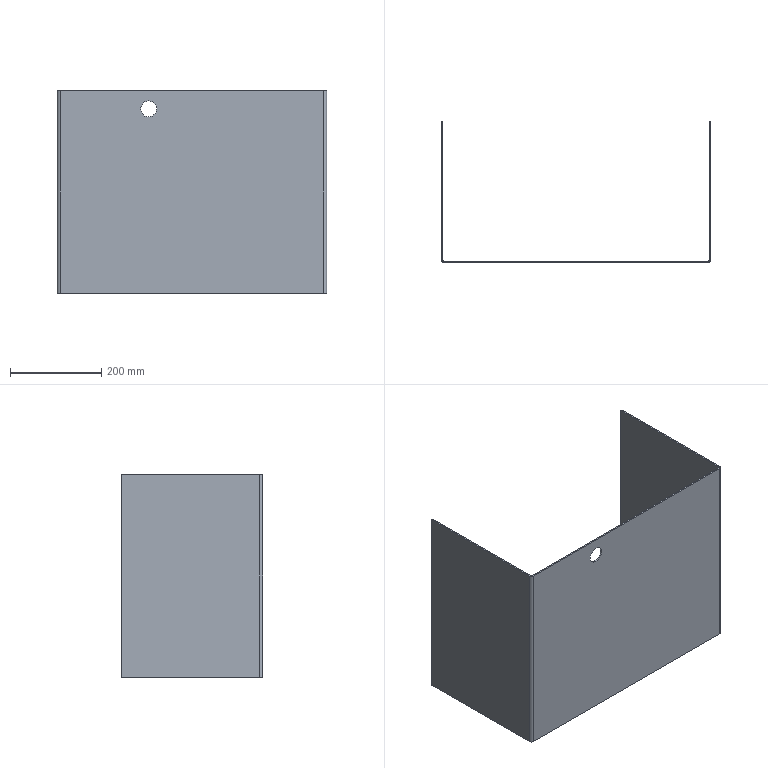Part | SolidWorks | features ICE 2, FlatPattern 1, SMBaseFlange 1, SheetMetal 1 | 1 solid | 28 faces | box 590 x 310 x 444 mm | volume 1595673 mm3 | plane 18 | cylinder 10 | commonest cylinder face diameters 6 x6 12 x2 35 x2
STEP:
#1=CARTESIAN_POINT('',(200.,0.,386.5));
#2=VERTEX_POINT('',#1);
#3=CARTESIAN_POINT('',(200.,0.,421.5));
#4=VERTEX_POINT('',#3);
#5=CARTESIAN_POINT('',(200.,0.,404.));
#6=DIRECTION('',(0.,1.,0.));
#7=DIRECTION('',(0.,0.,1.));
#8=AXIS2_PLACEMENT_3D('',#5,#6,#7);
#9=CIRCLE('',#8,17.5);
#10=EDGE_CURVE('',#2,#4,#9,.T.);
#11=ORIENTED_EDGE('',*,*,#10,.F.);
#12=CARTESIAN_POINT('',(200.,3.,386.5));
#13=VERTEX_POINT('',#12);
#14=CARTESIAN_POINT('',(200.,-7.,386.5));
#15=DIRECTION('',(0.,1.,0.));
#16=VECTOR('',#15,1000.);
#17=LINE('',#14,#16);
#18=EDGE_CURVE('',#2,#13,#17,.T.);
#19=ORIENTED_EDGE('',*,*,#18,.T.);
#20=CARTESIAN_POINT('',(200.,3.,421.5));
#21=VERTEX_POINT('',#20);
#22=CARTESIAN_POINT('',(200.,3.,404.));
#23=DIRECTION('',(0.,1.,0.));
#24=DIRECTION('',(0.,0.,1.));
#25=AXIS2_PLACEMENT_3D('',#22,#23,#24);
#26=CIRCLE('',#25,17.5);
#27=EDGE_CURVE('',#13,#21,#26,.T.);
#28=ORIENTED_EDGE('',*,*,#27,.T.);
#29=CARTESIAN_POINT('',(200.,-7.,421.5));
#30=DIRECTION('',(0.,1.,0.));
#31=VECTOR('',#30,1000.);
#32=LINE('',#29,#31);
#33=EDGE_CURVE('',#4,#21,#32,.T.);
#34=ORIENTED_EDGE('',*,*,#33,.F.);
#35=EDGE_LOOP('',(#11,#19,#28,#34));
#36=FACE_OUTER_BOUND('',#35,.T.);
#37=CARTESIAN_POINT('',(200.,-7.,404.));
#38=DIRECTION('',(0.,1.,0.));
#39=DIRECTION('',(0.,0.,1.));
#40=AXIS2_PLACEMENT_3D('',#37,#38,#39);
#41=CYLINDRICAL_SURFACE('',#40,17.5);
#42=ADVANCED_FACE('',(#36),#41,.F.);
#43=CARTESIAN_POINT('',(590.,307.,0.));
#44=VERTEX_POINT('',#43);
#45=CARTESIAN_POINT('',(590.,310.,3.));
#46=VERTEX_POINT('',#45);
#47=CARTESIAN_POINT('',(590.,307.,3.));
#48=DIRECTION('',(1.,0.,0.));
#49=DIRECTION('',(0.,0.,1.));
#50=AXIS2_PLACEMENT_3D('',#47,#48,#49);
#51=CIRCLE('',#50,3.);
#52=EDGE_CURVE('',#44,#46,#51,.T.);
#53=ORIENTED_EDGE('',*,*,#52,.T.);
#54=CARTESIAN_POINT('',(590.,310.,441.));
#55=VERTEX_POINT('',#54);
#56=CARTESIAN_POINT('',(590.,310.,444.));
#57=DIRECTION('',(0.,0.,-1.));
#58=VECTOR('',#57,1000.);
#59=LINE('',#56,#58);
#60=EDGE_CURVE('',#55,#46,#59,.T.);
#61=ORIENTED_EDGE('',*,*,#60,.F.);
#62=CARTESIAN_POINT('',(590.,307.,444.));
#63=VERTEX_POINT('',#62);
#64=CARTESIAN_POINT('',(590.,307.,441.));
#65=DIRECTION('',(1.,0.,0.));
#66=DIRECTION('',(0.,0.,1.));
#67=AXIS2_PLACEMENT_3D('',#64,#65,#66);
#68=CIRCLE('',#67,3.);
#69=EDGE_CURVE('',#55,#63,#68,.T.);
#70=ORIENTED_EDGE('',*,*,#69,.T.);
#71=CARTESIAN_POINT('',(590.,6.,444.));
#72=VERTEX_POINT('',#71);
#73=CARTESIAN_POINT('',(590.,0.,444.));
#74=DIRECTION('',(0.,1.,0.));
#75=VECTOR('',#74,1000.);
#76=LINE('',#73,#75);
#77=EDGE_CURVE('',#72,#63,#76,.T.);
#78=ORIENTED_EDGE('',*,*,#77,.F.);
#79=CARTESIAN_POINT('',(590.,6.,0.));
#80=VERTEX_POINT('',#79);
#81=CARTESIAN_POINT('',(590.,6.,444.));
#82=DIRECTION('',(0.,0.,-1.));
#83=VECTOR('',#82,1000.);
#84=LINE('',#81,#83);
#85=EDGE_CURVE('',#72,#80,#84,.T.);
#86=ORIENTED_EDGE('',*,*,#85,.T.);
#87=CARTESIAN_POINT('',(590.,0.,0.));
#88=DIRECTION('',(0.,1.,0.));
#89=VECTOR('',#88,1000.);
#90=LINE('',#87,#89);
#91=EDGE_CURVE('',#80,#44,#90,.T.);
#92=ORIENTED_EDGE('',*,*,#91,.T.);
#93=EDGE_LOOP('',(#53,#61,#70,#78,#86,#92));
#94=FACE_OUTER_BOUND('',#93,.T.);
#95=CARTESIAN_POINT('',(590.,0.,444.));
#96=DIRECTION('',(-1.,0.,0.));
#97=DIRECTION('',(0.,0.,1.));
#98=AXIS2_PLACEMENT_3D('',#95,#96,#97);
#99=PLANE('',#98);
#100=ADVANCED_FACE('',(#94),#99,.F.);
#101=CARTESIAN_POINT('',(587.,310.,441.));
#102=VERTEX_POINT('',#101);
#103=CARTESIAN_POINT('',(587.,310.,3.));
#104=VERTEX_POINT('',#103);
#105=CARTESIAN_POINT('',(587.,310.,444.));
#106=DIRECTION('',(0.,0.,-1.));
#107=VECTOR('',#106,1000.);
#108=LINE('',#105,#107);
#109=EDGE_CURVE('',#102,#104,#108,.T.);
#110=ORIENTED_EDGE('',*,*,#109,.T.);
#111=CARTESIAN_POINT('',(587.,307.,0.));
#112=VERTEX_POINT('',#111);
#113=CARTESIAN_POINT('',(587.,307.,3.));
#114=DIRECTION('',(1.,0.,0.));
#115=DIRECTION('',(0.,0.,1.));
#116=AXIS2_PLACEMENT_3D('',#113,#114,#115);
#117=CIRCLE('',#116,3.);
#118=EDGE_CURVE('',#112,#104,#117,.T.);
#119=ORIENTED_EDGE('',*,*,#118,.F.);
#120=CARTESIAN_POINT('',(587.,6.,0.));
#121=VERTEX_POINT('',#120);
#122=CARTESIAN_POINT('',(587.,0.,0.));
#123=DIRECTION('',(0.,1.,0.));
#124=VECTOR('',#123,1000.);
#125=LINE('',#122,#124);
#126=EDGE_CURVE('',#121,#112,#125,.T.);
#127=ORIENTED_EDGE('',*,*,#126,.F.);
#128=CARTESIAN_POINT('',(587.,6.,444.));
#129=VERTEX_POINT('',#128);
#130=CARTESIAN_POINT('',(587.,6.,444.));
#131=DIRECTION('',(0.,0.,-1.));
#132=VECTOR('',#131,1000.);
#133=LINE('',#130,#132);
#134=EDGE_CURVE('',#129,#121,#133,.T.);
#135=ORIENTED_EDGE('',*,*,#134,.F.);
#136=CARTESIAN_POINT('',(587.,307.,444.));
#137=VERTEX_POINT('',#136);
#138=CARTESIAN_POINT('',(587.,0.,444.));
#139=DIRECTION('',(0.,1.,0.));
#140=VECTOR('',#139,1000.);
#141=LINE('',#138,#140);
#142=EDGE_CURVE('',#129,#137,#141,.T.);
#143=ORIENTED_EDGE('',*,*,#142,.T.);
#144=CARTESIAN_POINT('',(587.,307.,441.));
#145=DIRECTION('',(1.,0.,0.));
#146=DIRECTION('',(0.,0.,1.));
#147=AXIS2_PLACEMENT_3D('',#144,#145,#146);
#148=CIRCLE('',#147,3.);
#149=EDGE_CURVE('',#102,#137,#148,.T.);
#150=ORIENTED_EDGE('',*,*,#149,.F.);
#151=EDGE_LOOP('',(#110,#119,#127,#135,#143,#150));
#152=FACE_OUTER_BOUND('',#151,.T.);
#153=CARTESIAN_POINT('',(587.,0.,444.));
#154=DIRECTION('',(-1.,0.,0.));
#155=DIRECTION('',(0.,0.,1.));
#156=AXIS2_PLACEMENT_3D('',#153,#154,#155);
#157=PLANE('',#156);
#158=ADVANCED_FACE('',(#152),#157,.T.);
#159=ORIENTED_EDGE('',*,*,#60,.T.);
#160=CARTESIAN_POINT('',(587.,310.,3.));
#161=DIRECTION('',(1.,0.,0.));
#162=VECTOR('',#161,1000.);
#163=LINE('',#160,#162);
#164=EDGE_CURVE('',#104,#46,#163,.T.);
#165=ORIENTED_EDGE('',*,*,#164,.F.);
#166=ORIENTED_EDGE('',*,*,#109,.F.);
#167=CARTESIAN_POINT('',(587.,310.,441.));
#168=DIRECTION('',(1.,0.,0.));
#169=VECTOR('',#168,1000.);
#170=LINE('',#167,#169);
#171=EDGE_CURVE('',#102,#55,#170,.T.);
#172=ORIENTED_EDGE('',*,*,#171,.T.);
#173=EDGE_LOOP('',(#159,#165,#166,#172));
#174=FACE_OUTER_BOUND('',#173,.T.);
#175=CARTESIAN_POINT('',(587.,310.,444.));
#176=DIRECTION('',(0.,1.,0.));
#177=DIRECTION('',(0.,0.,1.));
#178=AXIS2_PLACEMENT_3D('',#175,#176,#177);
#179=PLANE('',#178);
#180=ADVANCED_FACE('',(#174),#179,.T.);
#181=CARTESIAN_POINT('',(3.,307.,0.));
#182=VERTEX_POINT('',#181);
#183=CARTESIAN_POINT('',(3.,6.,0.));
#184=VERTEX_POINT('',#183);
#185=CARTESIAN_POINT('',(3.,0.,0.));
#186=DIRECTION('',(0.,-1.,0.));
#187=VECTOR('',#186,1000.);
#188=LINE('',#185,#187);
#189=EDGE_CURVE('',#182,#184,#188,.T.);
#190=ORIENTED_EDGE('',*,*,#189,.F.);
#191=CARTESIAN_POINT('',(3.,310.,3.));
#192=VERTEX_POINT('',#191);
#193=CARTESIAN_POINT('',(3.,307.,3.));
#194=DIRECTION('',(-1.,0.,0.));
#195=DIRECTION('',(0.,0.,-1.));
#196=AXIS2_PLACEMENT_3D('',#193,#194,#195);
#197=CIRCLE('',#196,3.);
#198=EDGE_CURVE('',#192,#182,#197,.T.);
#199=ORIENTED_EDGE('',*,*,#198,.F.);
#200=CARTESIAN_POINT('',(3.,310.,441.));
#201=VERTEX_POINT('',#200);
#202=CARTESIAN_POINT('',(3.,310.,444.));
#203=DIRECTION('',(0.,0.,-1.));
#204=VECTOR('',#203,1000.);
#205=LINE('',#202,#204);
#206=EDGE_CURVE('',#201,#192,#205,.T.);
#207=ORIENTED_EDGE('',*,*,#206,.F.);
#208=CARTESIAN_POINT('',(3.,307.,444.));
#209=VERTEX_POINT('',#208);
#210=CARTESIAN_POINT('',(3.,307.,441.));
#211=DIRECTION('',(-1.,0.,0.));
#212=DIRECTION('',(0.,0.,-1.));
#213=AXIS2_PLACEMENT_3D('',#210,#211,#212);
#214=CIRCLE('',#213,3.);
#215=EDGE_CURVE('',#209,#201,#214,.T.);
#216=ORIENTED_EDGE('',*,*,#215,.F.);
#217=CARTESIAN_POINT('',(3.,6.,444.));
#218=VERTEX_POINT('',#217);
#219=CARTESIAN_POINT('',(3.,0.,444.));
#220=DIRECTION('',(0.,-1.,0.));
#221=VECTOR('',#220,1000.);
#222=LINE('',#219,#221);
#223=EDGE_CURVE('',#209,#218,#222,.T.);
#224=ORIENTED_EDGE('',*,*,#223,.T.);
#225=CARTESIAN_POINT('',(3.,6.,444.));
#226=DIRECTION('',(0.,0.,-1.));
#227=VECTOR('',#226,1000.);
#228=LINE('',#225,#227);
#229=EDGE_CURVE('',#218,#184,#228,.T.);
#230=ORIENTED_EDGE('',*,*,#229,.T.);
#231=EDGE_LOOP('',(#190,#199,#207,#216,#224,#230));
#232=FACE_OUTER_BOUND('',#231,.T.);
#233=CARTESIAN_POINT('',(3.,0.,444.));
#234=DIRECTION('',(1.,0.,0.));
#235=DIRECTION('',(0.,0.,-1.));
#236=AXIS2_PLACEMENT_3D('',#233,#234,#235);
#237=PLANE('',#236);
#238=ADVANCED_FACE('',(#232),#237,.T.);
#239=CARTESIAN_POINT('',(0.,310.,3.));
#240=VERTEX_POINT('',#239);
#241=CARTESIAN_POINT('',(0.,307.,0.));
#242=VERTEX_POINT('',#241);
#243=CARTESIAN_POINT('',(0.,307.,3.));
#244=DIRECTION('',(-1.,0.,0.));
#245=DIRECTION('',(0.,0.,-1.));
#246=AXIS2_PLACEMENT_3D('',#243,#244,#245);
#247=CIRCLE('',#246,3.);
#248=EDGE_CURVE('',#240,#242,#247,.T.);
#249=ORIENTED_EDGE('',*,*,#248,.T.);
#250=CARTESIAN_POINT('',(0.,6.,0.));
#251=VERTEX_POINT('',#250);
#252=CARTESIAN_POINT('',(0.,0.,0.));
#253=DIRECTION('',(0.,-1.,0.));
#254=VECTOR('',#253,1000.);
#255=LINE('',#252,#254);
#256=EDGE_CURVE('',#242,#251,#255,.T.);
#257=ORIENTED_EDGE('',*,*,#256,.T.);
#258=CARTESIAN_POINT('',(0.,6.,444.));
#259=VERTEX_POINT('',#258);
#260=CARTESIAN_POINT('',(0.,6.,444.));
#261=DIRECTION('',(0.,0.,-1.));
#262=VECTOR('',#261,1000.);
#263=LINE('',#260,#262);
#264=EDGE_CURVE('',#259,#251,#263,.T.);
#265=ORIENTED_EDGE('',*,*,#264,.F.);
#266=CARTESIAN_POINT('',(0.,307.,444.));
#267=VERTEX_POINT('',#266);
#268=CARTESIAN_POINT('',(0.,0.,444.));
#269=DIRECTION('',(0.,-1.,0.));
#270=VECTOR('',#269,1000.);
#271=LINE('',#268,#270);
#272=EDGE_CURVE('',#267,#259,#271,.T.);
#273=ORIENTED_EDGE('',*,*,#272,.F.);
#274=CARTESIAN_POINT('',(0.,310.,441.));
#275=VERTEX_POINT('',#274);
#276=CARTESIAN_POINT('',(0.,307.,441.));
#277=DIRECTION('',(-1.,0.,0.));
#278=DIRECTION('',(0.,0.,-1.));
#279=AXIS2_PLACEMENT_3D('',#276,#277,#278);
#280=CIRCLE('',#279,3.);
#281=EDGE_CURVE('',#267,#275,#280,.T.);
#282=ORIENTED_EDGE('',*,*,#281,.T.);
#283=CARTESIAN_POINT('',(0.,310.,444.));
#284=DIRECTION('',(0.,0.,-1.));
#285=VECTOR('',#284,1000.);
#286=LINE('',#283,#285);
#287=EDGE_CURVE('',#275,#240,#286,.T.);
#288=ORIENTED_EDGE('',*,*,#287,.T.);
#289=EDGE_LOOP('',(#249,#257,#265,#273,#282,#288));
#290=FACE_OUTER_BOUND('',#289,.T.);
#291=CARTESIAN_POINT('',(0.,0.,444.));
#292=DIRECTION('',(1.,0.,0.));
#293=DIRECTION('',(0.,0.,-1.));
#294=AXIS2_PLACEMENT_3D('',#291,#292,#293);
#295=PLANE('',#294);
#296=ADVANCED_FACE('',(#290),#295,.F.);
#297=ORIENTED_EDGE('',*,*,#77,.T.);
#298=CARTESIAN_POINT('',(587.,307.,444.));
#299=DIRECTION('',(1.,0.,0.));
#300=VECTOR('',#299,1000.);
#301=LINE('',#298,#300);
#302=EDGE_CURVE('',#137,#63,#301,.T.);
#303=ORIENTED_EDGE('',*,*,#302,.F.);
#304=ORIENTED_EDGE('',*,*,#142,.F.);
#305=CARTESIAN_POINT('',(587.,6.,444.));
#306=DIRECTION('',(1.,0.,0.));
#307=VECTOR('',#306,1000.);
#308=LINE('',#305,#307);
#309=EDGE_CURVE('',#129,#72,#308,.T.);
#310=ORIENTED_EDGE('',*,*,#309,.T.);
#311=EDGE_LOOP('',(#297,#303,#304,#310));
#312=FACE_OUTER_BOUND('',#311,.T.);
#313=CARTESIAN_POINT('',(584.,6.,444.));
#314=DIRECTION('',(0.,0.,1.));
#315=DIRECTION('',(1.,0.,0.));
#316=AXIS2_PLACEMENT_3D('',#313,#314,#315);
#317=PLANE('',#316);
#318=ADVANCED_FACE('',(#312),#317,.T.);
#319=CARTESIAN_POINT('',(3.,310.,3.));
#320=DIRECTION('',(-1.,0.,0.));
#321=VECTOR('',#320,1000.);
#322=LINE('',#319,#321);
#323=EDGE_CURVE('',#192,#240,#322,.T.);
#324=ORIENTED_EDGE('',*,*,#323,.T.);
#325=ORIENTED_EDGE('',*,*,#287,.F.);
#326=CARTESIAN_POINT('',(3.,310.,441.));
#327=DIRECTION('',(-1.,0.,0.));
#328=VECTOR('',#327,1000.);
#329=LINE('',#326,#328);
#330=EDGE_CURVE('',#201,#275,#329,.T.);
#331=ORIENTED_EDGE('',*,*,#330,.F.);
#332=ORIENTED_EDGE('',*,*,#206,.T.);
#333=EDGE_LOOP('',(#324,#325,#331,#332));
#334=FACE_OUTER_BOUND('',#333,.T.);
#335=CARTESIAN_POINT('',(0.,310.,444.));
#336=DIRECTION('',(0.,1.,0.));
#337=DIRECTION('',(0.,0.,1.));
#338=AXIS2_PLACEMENT_3D('',#335,#336,#337);
#339=PLANE('',#338);
#340=ADVANCED_FACE('',(#334),#339,.T.);
#341=CARTESIAN_POINT('',(0.,6.,444.));
#342=DIRECTION('',(1.,0.,0.));
#343=VECTOR('',#342,1000.);
#344=LINE('',#341,#343);
#345=EDGE_CURVE('',#259,#218,#344,.T.);
#346=ORIENTED_EDGE('',*,*,#345,.F.);
#347=CARTESIAN_POINT('',(6.,0.,444.));
#348=VERTEX_POINT('',#347);
#349=CARTESIAN_POINT('',(6.,6.,444.));
#350=DIRECTION('',(0.,0.,1.));
#351=DIRECTION('',(-1.,0.,0.));
#352=AXIS2_PLACEMENT_3D('',#349,#350,#351);
#353=CIRCLE('',#352,6.);
#354=EDGE_CURVE('',#259,#348,#353,.T.);
#355=ORIENTED_EDGE('',*,*,#354,.T.);
#356=CARTESIAN_POINT('',(6.,3.,444.));
#357=VERTEX_POINT('',#356);
#358=CARTESIAN_POINT('',(6.,3.,444.));
#359=DIRECTION('',(0.,-1.,0.));
#360=VECTOR('',#359,1000.);
#361=LINE('',#358,#360);
#362=EDGE_CURVE('',#357,#348,#361,.T.);
#363=ORIENTED_EDGE('',*,*,#362,.F.);
#364=CARTESIAN_POINT('',(6.,6.,444.));
#365=DIRECTION('',(0.,0.,1.));
#366=DIRECTION('',(1.,0.,0.));
#367=AXIS2_PLACEMENT_3D('',#364,#365,#366);
#368=CIRCLE('',#367,3.);
#369=EDGE_CURVE('',#218,#357,#368,.T.);
#370=ORIENTED_EDGE('',*,*,#369,.F.);
#371=EDGE_LOOP('',(#346,#355,#363,#370));
#372=FACE_OUTER_BOUND('',#371,.T.);
#373=CARTESIAN_POINT('',(0.,6.,444.));
#374=DIRECTION('',(0.,0.,1.));
#375=DIRECTION('',(1.,0.,0.));
#376=AXIS2_PLACEMENT_3D('',#373,#374,#375);
#377=PLANE('',#376);
#378=ADVANCED_FACE('',(#372),#377,.T.);
#379=CARTESIAN_POINT('',(3.,307.,444.));
#380=DIRECTION('',(-1.,0.,0.));
#381=VECTOR('',#380,1000.);
#382=LINE('',#379,#381);
#383=EDGE_CURVE('',#209,#267,#382,.T.);
#384=ORIENTED_EDGE('',*,*,#383,.T.);
#385=ORIENTED_EDGE('',*,*,#272,.T.);
#386=ORIENTED_EDGE('',*,*,#345,.T.);
#387=ORIENTED_EDGE('',*,*,#223,.F.);
#388=EDGE_LOOP('',(#384,#385,#386,#387));
#389=FACE_OUTER_BOUND('',#388,.T.);
#390=CARTESIAN_POINT('',(6.,3.,444.));
#391=DIRECTION('',(0.,0.,1.));
#392=DIRECTION('',(1.,0.,0.));
#393=AXIS2_PLACEMENT_3D('',#390,#391,#392);
#394=PLANE('',#393);
#395=ADVANCED_FACE('',(#389),#394,.T.);
#396=CARTESIAN_POINT('',(6.,0.,0.));
#397=VERTEX_POINT('',#396);
#398=CARTESIAN_POINT('',(6.,3.,0.));
#399=VERTEX_POINT('',#398);
#400=CARTESIAN_POINT('',(6.,0.,0.));
#401=DIRECTION('',(0.,1.,0.));
#402=VECTOR('',#401,1000.);
#403=LINE('',#400,#402);
#404=EDGE_CURVE('',#397,#399,#403,.T.);
#405=ORIENTED_EDGE('',*,*,#404,.F.);
#406=CARTESIAN_POINT('',(6.,6.,0.));
#407=DIRECTION('',(0.,0.,1.));
#408=DIRECTION('',(-1.,0.,0.));
#409=AXIS2_PLACEMENT_3D('',#406,#407,#408);
#410=CIRCLE('',#409,6.);
#411=EDGE_CURVE('',#251,#397,#410,.T.);
#412=ORIENTED_EDGE('',*,*,#411,.F.);
#413=CARTESIAN_POINT('',(3.,6.,0.));
#414=DIRECTION('',(-1.,0.,0.));
#415=VECTOR('',#414,1000.);
#416=LINE('',#413,#415);
#417=EDGE_CURVE('',#184,#251,#416,.T.);
#418=ORIENTED_EDGE('',*,*,#417,.F.);
#419=CARTESIAN_POINT('',(6.,6.,0.));
#420=DIRECTION('',(0.,0.,1.));
#421=DIRECTION('',(1.,0.,0.));
#422=AXIS2_PLACEMENT_3D('',#419,#420,#421);
#423=CIRCLE('',#422,3.);
#424=EDGE_CURVE('',#184,#399,#423,.T.);
#425=ORIENTED_EDGE('',*,*,#424,.T.);
#426=EDGE_LOOP('',(#405,#412,#418,#425));
#427=FACE_OUTER_BOUND('',#426,.T.);
#428=CARTESIAN_POINT('',(6.,0.,0.));
#429=DIRECTION('',(0.,0.,-1.));
#430=DIRECTION('',(-1.,0.,0.));
#431=AXIS2_PLACEMENT_3D('',#428,#429,#430);
#432=PLANE('',#431);
#433=ADVANCED_FACE('',(#427),#432,.T.);
#434=CARTESIAN_POINT('',(584.,0.,0.));
#435=VERTEX_POINT('',#434);
#436=CARTESIAN_POINT('',(0.,0.,0.));
#437=DIRECTION('',(1.,0.,0.));
#438=VECTOR('',#437,1000.);
#439=LINE('',#436,#438);
#440=EDGE_CURVE('',#397,#435,#439,.T.);
#441=ORIENTED_EDGE('',*,*,#440,.F.);
#442=ORIENTED_EDGE('',*,*,#404,.T.);
#443=CARTESIAN_POINT('',(584.,3.,0.));
#444=VERTEX_POINT('',#443);
#445=CARTESIAN_POINT('',(0.,3.,0.));
#446=DIRECTION('',(1.,0.,0.));
#447=VECTOR('',#446,1000.);
#448=LINE('',#445,#447);
#449=EDGE_CURVE('',#399,#444,#448,.T.);
#450=ORIENTED_EDGE('',*,*,#449,.T.);
#451=CARTESIAN_POINT('',(584.,3.,0.));
#452=DIRECTION('',(0.,-1.,0.));
#453=VECTOR('',#452,1000.);
#454=LINE('',#451,#453);
#455=EDGE_CURVE('',#444,#435,#454,.T.);
#456=ORIENTED_EDGE('',*,*,#455,.T.);
#457=EDGE_LOOP('',(#441,#442,#450,#456));
#458=FACE_OUTER_BOUND('',#457,.T.);
#459=CARTESIAN_POINT('',(3.,6.,0.));
#460=DIRECTION('',(0.,0.,-1.));
#461=DIRECTION('',(-1.,0.,0.));
#462=AXIS2_PLACEMENT_3D('',#459,#460,#461);
#463=PLANE('',#462);
#464=ADVANCED_FACE('',(#458),#463,.T.);
#465=CARTESIAN_POINT('',(584.,0.,444.));
#466=VERTEX_POINT('',#465);
#467=CARTESIAN_POINT('',(584.,3.,444.));
#468=VERTEX_POINT('',#467);
#469=CARTESIAN_POINT('',(584.,0.,444.));
#470=DIRECTION('',(0.,1.,0.));
#471=VECTOR('',#470,1000.);
#472=LINE('',#469,#471);
#473=EDGE_CURVE('',#466,#468,#472,.T.);
#474=ORIENTED_EDGE('',*,*,#473,.F.);
#475=CARTESIAN_POINT('',(584.,6.,444.));
#476=DIRECTION('',(0.,0.,1.));
#477=DIRECTION('',(-1.,0.,0.));
#478=AXIS2_PLACEMENT_3D('',#475,#476,#477);
#479=CIRCLE('',#478,6.);
#480=EDGE_CURVE('',#466,#72,#479,.T.);
#481=ORIENTED_EDGE('',*,*,#480,.T.);
#482=ORIENTED_EDGE('',*,*,#309,.F.);
#483=CARTESIAN_POINT('',(584.,6.,444.));
#484=DIRECTION('',(0.,0.,1.));
#485=DIRECTION('',(1.,0.,0.));
#486=AXIS2_PLACEMENT_3D('',#483,#484,#485);
#487=CIRCLE('',#486,3.);
#488=EDGE_CURVE('',#468,#129,#487,.T.);
#489=ORIENTED_EDGE('',*,*,#488,.F.);
#490=EDGE_LOOP('',(#474,#481,#482,#489));
#491=FACE_OUTER_BOUND('',#490,.T.);
#492=CARTESIAN_POINT('',(584.,0.,444.));
#493=DIRECTION('',(0.,0.,1.));
#494=DIRECTION('',(1.,0.,0.));
#495=AXIS2_PLACEMENT_3D('',#492,#493,#494);
#496=PLANE('',#495);
#497=ADVANCED_FACE('',(#491),#496,.T.);
#498=CARTESIAN_POINT('',(0.,0.,444.));
#499=DIRECTION('',(1.,0.,0.));
#500=VECTOR('',#499,1000.);
#501=LINE('',#498,#500);
#502=EDGE_CURVE('',#348,#466,#501,.T.);
#503=ORIENTED_EDGE('',*,*,#502,.T.);
#504=ORIENTED_EDGE('',*,*,#473,.T.);
#505=CARTESIAN_POINT('',(0.,3.,444.));
#506=DIRECTION('',(1.,0.,0.));
#507=VECTOR('',#506,1000.);
#508=LINE('',#505,#507);
#509=EDGE_CURVE('',#357,#468,#508,.T.);
#510=ORIENTED_EDGE('',*,*,#509,.F.);
#511=ORIENTED_EDGE('',*,*,#362,.T.);
#512=EDGE_LOOP('',(#503,#504,#510,#511));
#513=FACE_OUTER_BOUND('',#512,.T.);
#514=CARTESIAN_POINT('',(587.,6.,444.));
#515=DIRECTION('',(0.,0.,1.));
#516=DIRECTION('',(1.,0.,0.));
#517=AXIS2_PLACEMENT_3D('',#514,#515,#516);
#518=PLANE('',#517);
#519=ADVANCED_FACE('',(#513),#518,.T.);
#520=CARTESIAN_POINT('',(590.,6.,0.));
#521=DIRECTION('',(-1.,0.,0.));
#522=VECTOR('',#521,1000.);
#523=LINE('',#520,#522);
#524=EDGE_CURVE('',#80,#121,#523,.T.);
#525=ORIENTED_EDGE('',*,*,#524,.F.);
#526=CARTESIAN_POINT('',(584.,6.,0.));
#527=DIRECTION('',(0.,0.,1.));
#528=DIRECTION('',(-1.,0.,0.));
#529=AXIS2_PLACEMENT_3D('',#526,#527,#528);
#530=CIRCLE('',#529,6.);
#531=EDGE_CURVE('',#435,#80,#530,.T.);
#532=ORIENTED_EDGE('',*,*,#531,.F.);
#533=ORIENTED_EDGE('',*,*,#455,.F.);
#534=CARTESIAN_POINT('',(584.,6.,0.));
#535=DIRECTION('',(0.,0.,1.));
#536=DIRECTION('',(1.,0.,0.));
#537=AXIS2_PLACEMENT_3D('',#534,#535,#536);
#538=CIRCLE('',#537,3.);
#539=EDGE_CURVE('',#444,#121,#538,.T.);
#540=ORIENTED_EDGE('',*,*,#539,.T.);
#541=EDGE_LOOP('',(#525,#532,#533,#540));
#542=FACE_OUTER_BOUND('',#541,.T.);
#543=CARTESIAN_POINT('',(590.,6.,0.));
#544=DIRECTION('',(0.,0.,-1.));
#545=DIRECTION('',(-1.,0.,0.));
#546=AXIS2_PLACEMENT_3D('',#543,#544,#545);
#547=PLANE('',#546);
#548=ADVANCED_FACE('',(#542),#547,.T.);
#549=CARTESIAN_POINT('',(587.,307.,0.));
#550=DIRECTION('',(1.,0.,0.));
#551=VECTOR('',#550,1000.);
#552=LINE('',#549,#551);
#553=EDGE_CURVE('',#112,#44,#552,.T.);
#554=ORIENTED_EDGE('',*,*,#553,.T.);
#555=ORIENTED_EDGE('',*,*,#91,.F.);
#556=ORIENTED_EDGE('',*,*,#524,.T.);
#557=ORIENTED_EDGE('',*,*,#126,.T.);
#558=EDGE_LOOP('',(#554,#555,#556,#557));
#559=FACE_OUTER_BOUND('',#558,.T.);
#560=CARTESIAN_POINT('',(584.,3.,0.));
#561=DIRECTION('',(0.,0.,-1.));
#562=DIRECTION('',(-1.,0.,0.));
#563=AXIS2_PLACEMENT_3D('',#560,#561,#562);
#564=PLANE('',#563);
#565=ADVANCED_FACE('',(#559),#564,.T.);
#566=ORIENTED_EDGE('',*,*,#539,.F.);
#567=CARTESIAN_POINT('',(584.,3.,444.));
#568=DIRECTION('',(0.,0.,-1.));
#569=VECTOR('',#568,1000.);
#570=LINE('',#567,#569);
#571=EDGE_CURVE('',#468,#444,#570,.T.);
#572=ORIENTED_EDGE('',*,*,#571,.F.);
#573=ORIENTED_EDGE('',*,*,#488,.T.);
#574=ORIENTED_EDGE('',*,*,#134,.T.);
#575=EDGE_LOOP('',(#566,#572,#573,#574));
#576=FACE_OUTER_BOUND('',#575,.T.);
#577=CARTESIAN_POINT('',(584.,6.,444.));
#578=DIRECTION('',(0.,0.,-1.));
#579=DIRECTION('',(-1.,0.,0.));
#580=AXIS2_PLACEMENT_3D('',#577,#578,#579);
#581=CYLINDRICAL_SURFACE('',#580,3.);
#582=ADVANCED_FACE('',(#576),#581,.F.);
#583=CARTESIAN_POINT('',(200.,3.,404.));
#584=DIRECTION('',(0.,1.,0.));
#585=DIRECTION('',(0.,0.,1.));
#586=AXIS2_PLACEMENT_3D('',#583,#584,#585);
#587=CIRCLE('',#586,17.5);
#588=EDGE_CURVE('',#21,#13,#587,.T.);
#589=ORIENTED_EDGE('',*,*,#588,.F.);
#590=ORIENTED_EDGE('',*,*,#27,.F.);
#591=EDGE_LOOP('',(#589,#590));
#592=FACE_BOUND('',#591,.T.);
#593=ORIENTED_EDGE('',*,*,#449,.F.);
#594=CARTESIAN_POINT('',(6.,3.,444.));
#595=DIRECTION('',(0.,0.,-1.));
#596=VECTOR('',#595,1000.);
#597=LINE('',#594,#596);
#598=EDGE_CURVE('',#357,#399,#597,.T.);
#599=ORIENTED_EDGE('',*,*,#598,.F.);
#600=ORIENTED_EDGE('',*,*,#509,.T.);
#601=ORIENTED_EDGE('',*,*,#571,.T.);
#602=EDGE_LOOP('',(#593,#599,#600,#601));
#603=FACE_OUTER_BOUND('',#602,.T.);
#604=CARTESIAN_POINT('',(0.,3.,444.));
#605=DIRECTION('',(0.,1.,0.));
#606=DIRECTION('',(0.,0.,1.));
#607=AXIS2_PLACEMENT_3D('',#604,#605,#606);
#608=PLANE('',#607);
#609=ADVANCED_FACE('',(#592,#603),#608,.T.);
#610=ORIENTED_EDGE('',*,*,#424,.F.);
#611=ORIENTED_EDGE('',*,*,#229,.F.);
#612=ORIENTED_EDGE('',*,*,#369,.T.);
#613=ORIENTED_EDGE('',*,*,#598,.T.);
#614=EDGE_LOOP('',(#610,#611,#612,#613));
#615=FACE_OUTER_BOUND('',#614,.T.);
#616=CARTESIAN_POINT('',(6.,6.,444.));
#617=DIRECTION('',(0.,0.,-1.));
#618=DIRECTION('',(-1.,0.,0.));
#619=AXIS2_PLACEMENT_3D('',#616,#617,#618);
#620=CYLINDRICAL_SURFACE('',#619,3.);
#621=ADVANCED_FACE('',(#615),#620,.F.);
#622=ORIENTED_EDGE('',*,*,#411,.T.);
#623=CARTESIAN_POINT('',(6.,0.,444.));
#624=DIRECTION('',(0.,0.,-1.));
#625=VECTOR('',#624,1000.);
#626=LINE('',#623,#625);
#627=EDGE_CURVE('',#348,#397,#626,.T.);
#628=ORIENTED_EDGE('',*,*,#627,.F.);
#629=ORIENTED_EDGE('',*,*,#354,.F.);
#630=ORIENTED_EDGE('',*,*,#264,.T.);
#631=EDGE_LOOP('',(#622,#628,#629,#630));
#632=FACE_OUTER_BOUND('',#631,.T.);
#633=CARTESIAN_POINT('',(6.,6.,444.));
#634=DIRECTION('',(0.,0.,-1.));
#635=DIRECTION('',(-1.,0.,0.));
#636=AXIS2_PLACEMENT_3D('',#633,#634,#635);
#637=CYLINDRICAL_SURFACE('',#636,6.);
#638=ADVANCED_FACE('',(#632),#637,.T.);
#639=CARTESIAN_POINT('',(200.,0.,404.));
#640=DIRECTION('',(0.,1.,0.));
#641=DIRECTION('',(0.,0.,1.));
#642=AXIS2_PLACEMENT_3D('',#639,#640,#641);
#643=CIRCLE('',#642,17.5);
#644=EDGE_CURVE('',#4,#2,#643,.T.);
#645=ORIENTED_EDGE('',*,*,#644,.T.);
#646=ORIENTED_EDGE('',*,*,#10,.T.);
#647=EDGE_LOOP('',(#645,#646));
#648=FACE_BOUND('',#647,.T.);
#649=ORIENTED_EDGE('',*,*,#440,.T.);
#650=CARTESIAN_POINT('',(584.,0.,444.));
#651=DIRECTION('',(0.,0.,-1.));
#652=VECTOR('',#651,1000.);
#653=LINE('',#650,#652);
#654=EDGE_CURVE('',#466,#435,#653,.T.);
#655=ORIENTED_EDGE('',*,*,#654,.F.);
#656=ORIENTED_EDGE('',*,*,#502,.F.);
#657=ORIENTED_EDGE('',*,*,#627,.T.);
#658=EDGE_LOOP('',(#649,#655,#656,#657));
#659=FACE_OUTER_BOUND('',#658,.T.);
#660=CARTESIAN_POINT('',(0.,0.,444.));
#661=DIRECTION('',(0.,1.,0.));
#662=DIRECTION('',(0.,0.,1.));
#663=AXIS2_PLACEMENT_3D('',#660,#661,#662);
#664=PLANE('',#663);
#665=ADVANCED_FACE('',(#648,#659),#664,.F.);
#666=ORIENTED_EDGE('',*,*,#531,.T.);
#667=ORIENTED_EDGE('',*,*,#85,.F.);
#668=ORIENTED_EDGE('',*,*,#480,.F.);
#669=ORIENTED_EDGE('',*,*,#654,.T.);
#670=EDGE_LOOP('',(#666,#667,#668,#669));
#671=FACE_OUTER_BOUND('',#670,.T.);
#672=CARTESIAN_POINT('',(584.,6.,444.));
#673=DIRECTION('',(0.,0.,-1.));
#674=DIRECTION('',(-1.,0.,0.));
#675=AXIS2_PLACEMENT_3D('',#672,#673,#674);
#676=CYLINDRICAL_SURFACE('',#675,6.);
#677=ADVANCED_FACE('',(#671),#676,.T.);
#678=ORIENTED_EDGE('',*,*,#256,.F.);
#679=CARTESIAN_POINT('',(3.,307.,0.));
#680=DIRECTION('',(-1.,0.,0.));
#681=VECTOR('',#680,1000.);
#682=LINE('',#679,#681);
#683=EDGE_CURVE('',#182,#242,#682,.T.);
#684=ORIENTED_EDGE('',*,*,#683,.F.);
#685=ORIENTED_EDGE('',*,*,#189,.T.);
#686=ORIENTED_EDGE('',*,*,#417,.T.);
#687=EDGE_LOOP('',(#678,#684,#685,#686));
#688=FACE_OUTER_BOUND('',#687,.T.);
#689=CARTESIAN_POINT('',(584.,6.,0.));
#690=DIRECTION('',(0.,0.,1.));
#691=DIRECTION('',(1.,0.,0.));
#692=AXIS2_PLACEMENT_3D('',#689,#690,#691);
#693=PLANE('',#692);
#694=ADVANCED_FACE('',(#688),#693,.F.);
#695=ORIENTED_EDGE('',*,*,#18,.F.);
#696=ORIENTED_EDGE('',*,*,#644,.F.);
#697=ORIENTED_EDGE('',*,*,#33,.T.);
#698=ORIENTED_EDGE('',*,*,#588,.T.);
#699=EDGE_LOOP('',(#695,#696,#697,#698));
#700=FACE_OUTER_BOUND('',#699,.T.);
#701=CARTESIAN_POINT('',(200.,-7.,404.));
#702=DIRECTION('',(0.,1.,0.));
#703=DIRECTION('',(0.,0.,1.));
#704=AXIS2_PLACEMENT_3D('',#701,#702,#703);
#705=CYLINDRICAL_SURFACE('',#704,17.5);
#706=ADVANCED_FACE('',(#700),#705,.F.);
#707=ORIENTED_EDGE('',*,*,#215,.T.);
#708=ORIENTED_EDGE('',*,*,#330,.T.);
#709=ORIENTED_EDGE('',*,*,#281,.F.);
#710=ORIENTED_EDGE('',*,*,#383,.F.);
#711=EDGE_LOOP('',(#707,#708,#709,#710));
#712=FACE_OUTER_BOUND('',#711,.T.);
#713=CARTESIAN_POINT('',(3.,307.,441.));
#714=DIRECTION('',(1.,0.,0.));
#715=DIRECTION('',(0.,0.,-1.));
#716=AXIS2_PLACEMENT_3D('',#713,#714,#715);
#717=CYLINDRICAL_SURFACE('',#716,3.);
#718=ADVANCED_FACE('',(#712),#717,.T.);
#719=ORIENTED_EDGE('',*,*,#149,.T.);
#720=ORIENTED_EDGE('',*,*,#302,.T.);
#721=ORIENTED_EDGE('',*,*,#69,.F.);
#722=ORIENTED_EDGE('',*,*,#171,.F.);
#723=EDGE_LOOP('',(#719,#720,#721,#722));
#724=FACE_OUTER_BOUND('',#723,.T.);
#725=CARTESIAN_POINT('',(587.,307.,441.));
#726=DIRECTION('',(-1.,0.,0.));
#727=DIRECTION('',(0.,0.,1.));
#728=AXIS2_PLACEMENT_3D('',#725,#726,#727);
#729=CYLINDRICAL_SURFACE('',#728,3.);
#730=ADVANCED_FACE('',(#724),#729,.T.);
#731=ORIENTED_EDGE('',*,*,#198,.T.);
#732=ORIENTED_EDGE('',*,*,#683,.T.);
#733=ORIENTED_EDGE('',*,*,#248,.F.);
#734=ORIENTED_EDGE('',*,*,#323,.F.);
#735=EDGE_LOOP('',(#731,#732,#733,#734));
#736=FACE_OUTER_BOUND('',#735,.T.);
#737=CARTESIAN_POINT('',(3.,307.,3.));
#738=DIRECTION('',(1.,0.,0.));
#739=DIRECTION('',(0.,0.,-1.));
#740=AXIS2_PLACEMENT_3D('',#737,#738,#739);
#741=CYLINDRICAL_SURFACE('',#740,3.);
#742=ADVANCED_FACE('',(#736),#741,.T.);
#743=ORIENTED_EDGE('',*,*,#118,.T.);
#744=ORIENTED_EDGE('',*,*,#164,.T.);
#745=ORIENTED_EDGE('',*,*,#52,.F.);
#746=ORIENTED_EDGE('',*,*,#553,.F.);
#747=EDGE_LOOP('',(#743,#744,#745,#746));
#748=FACE_OUTER_BOUND('',#747,.T.);
#749=CARTESIAN_POINT('',(587.,307.,3.));
#750=DIRECTION('',(-1.,0.,0.));
#751=DIRECTION('',(0.,0.,1.));
#752=AXIS2_PLACEMENT_3D('',#749,#750,#751);
#753=CYLINDRICAL_SURFACE('',#752,3.);
#754=ADVANCED_FACE('',(#748),#753,.T.);
#755=CLOSED_SHELL('',(#42,#100,#158,#180,#238,#296,#318,#340,#378,#395,#433,#464,#497,#519,#548,#565,#582,#609,#621,#638,#665,#677,#694,#706,#718,#730,#742,#754));
#756=MANIFOLD_SOLID_BREP('',#755);
#757=CARTESIAN_POINT('',(0.,0.,0.));
#758=DIRECTION('',(0.,0.,1.));
#759=DIRECTION('',(1.,0.,0.));
#760=AXIS2_PLACEMENT_3D('',#757,#758,#759);
#761=(LENGTH_UNIT()NAMED_UNIT(*)SI_UNIT(.MILLI.,.METRE.));
#762=UNCERTAINTY_MEASURE_WITH_UNIT(LENGTH_MEASURE(0.00001),#761,'','');
#763=(NAMED_UNIT(*)PLANE_ANGLE_UNIT()SI_UNIT($,.RADIAN.));
#764=(NAMED_UNIT(*)SI_UNIT($,.STERADIAN.)SOLID_ANGLE_UNIT());
#765=(GEOMETRIC_REPRESENTATION_CONTEXT(3)GLOBAL_UNCERTAINTY_ASSIGNED_CONTEXT((#762))GLOBAL_UNIT_ASSIGNED_CONTEXT((#761,#763,#764))REPRESENTATION_CONTEXT('',''));
#766=ADVANCED_BREP_SHAPE_REPRESENTATION('',(#756,#760),#765);